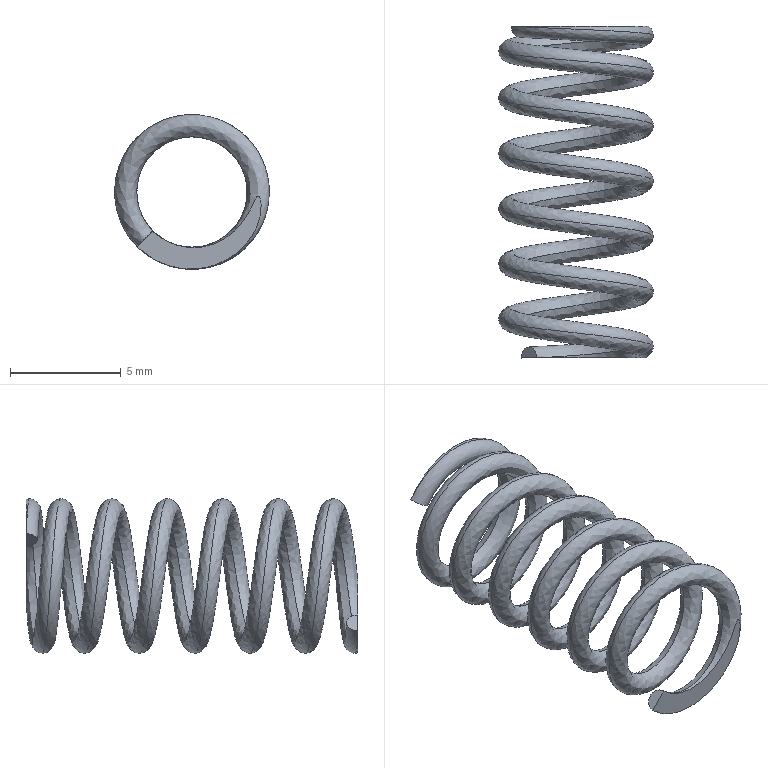Part | SolidWorks | features Helix 1, ICE 1, Sweep 1 | 1 solid | 6 faces | box 6.997 x 15.003 x 6.998 mm | volume 95.492 mm3 | plane 4 | spline 2